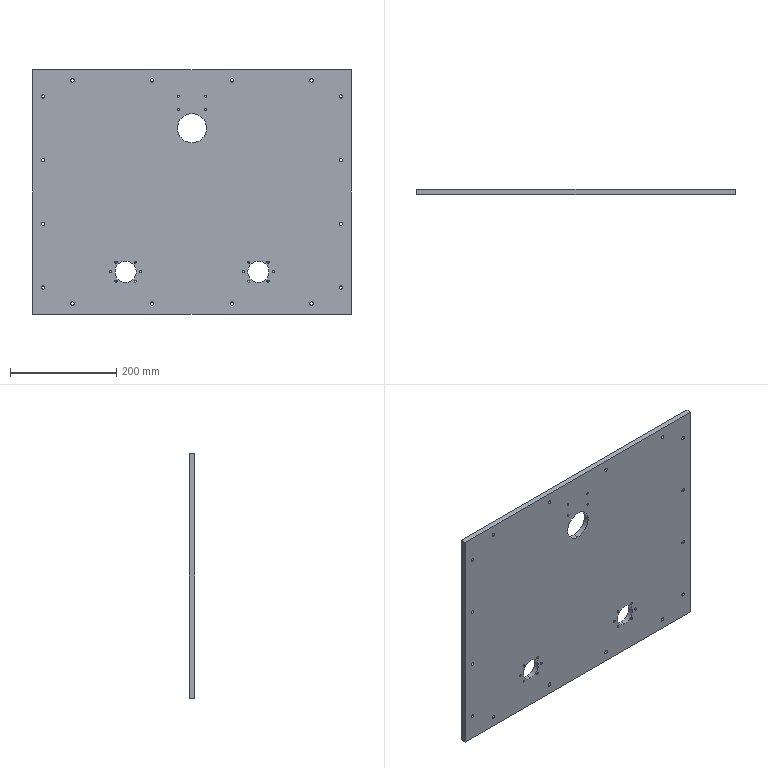Part | STEP file | Bracket二前立Plate | 1 solid | 108 faces | box 600 x 10 x 460 mm | volume 2701010 mm3 | cylinder 70 | cone 32 | plane 6 | commonest cylinder face diameters 4.2 x32 6.6 x32 40 x4 55 x2